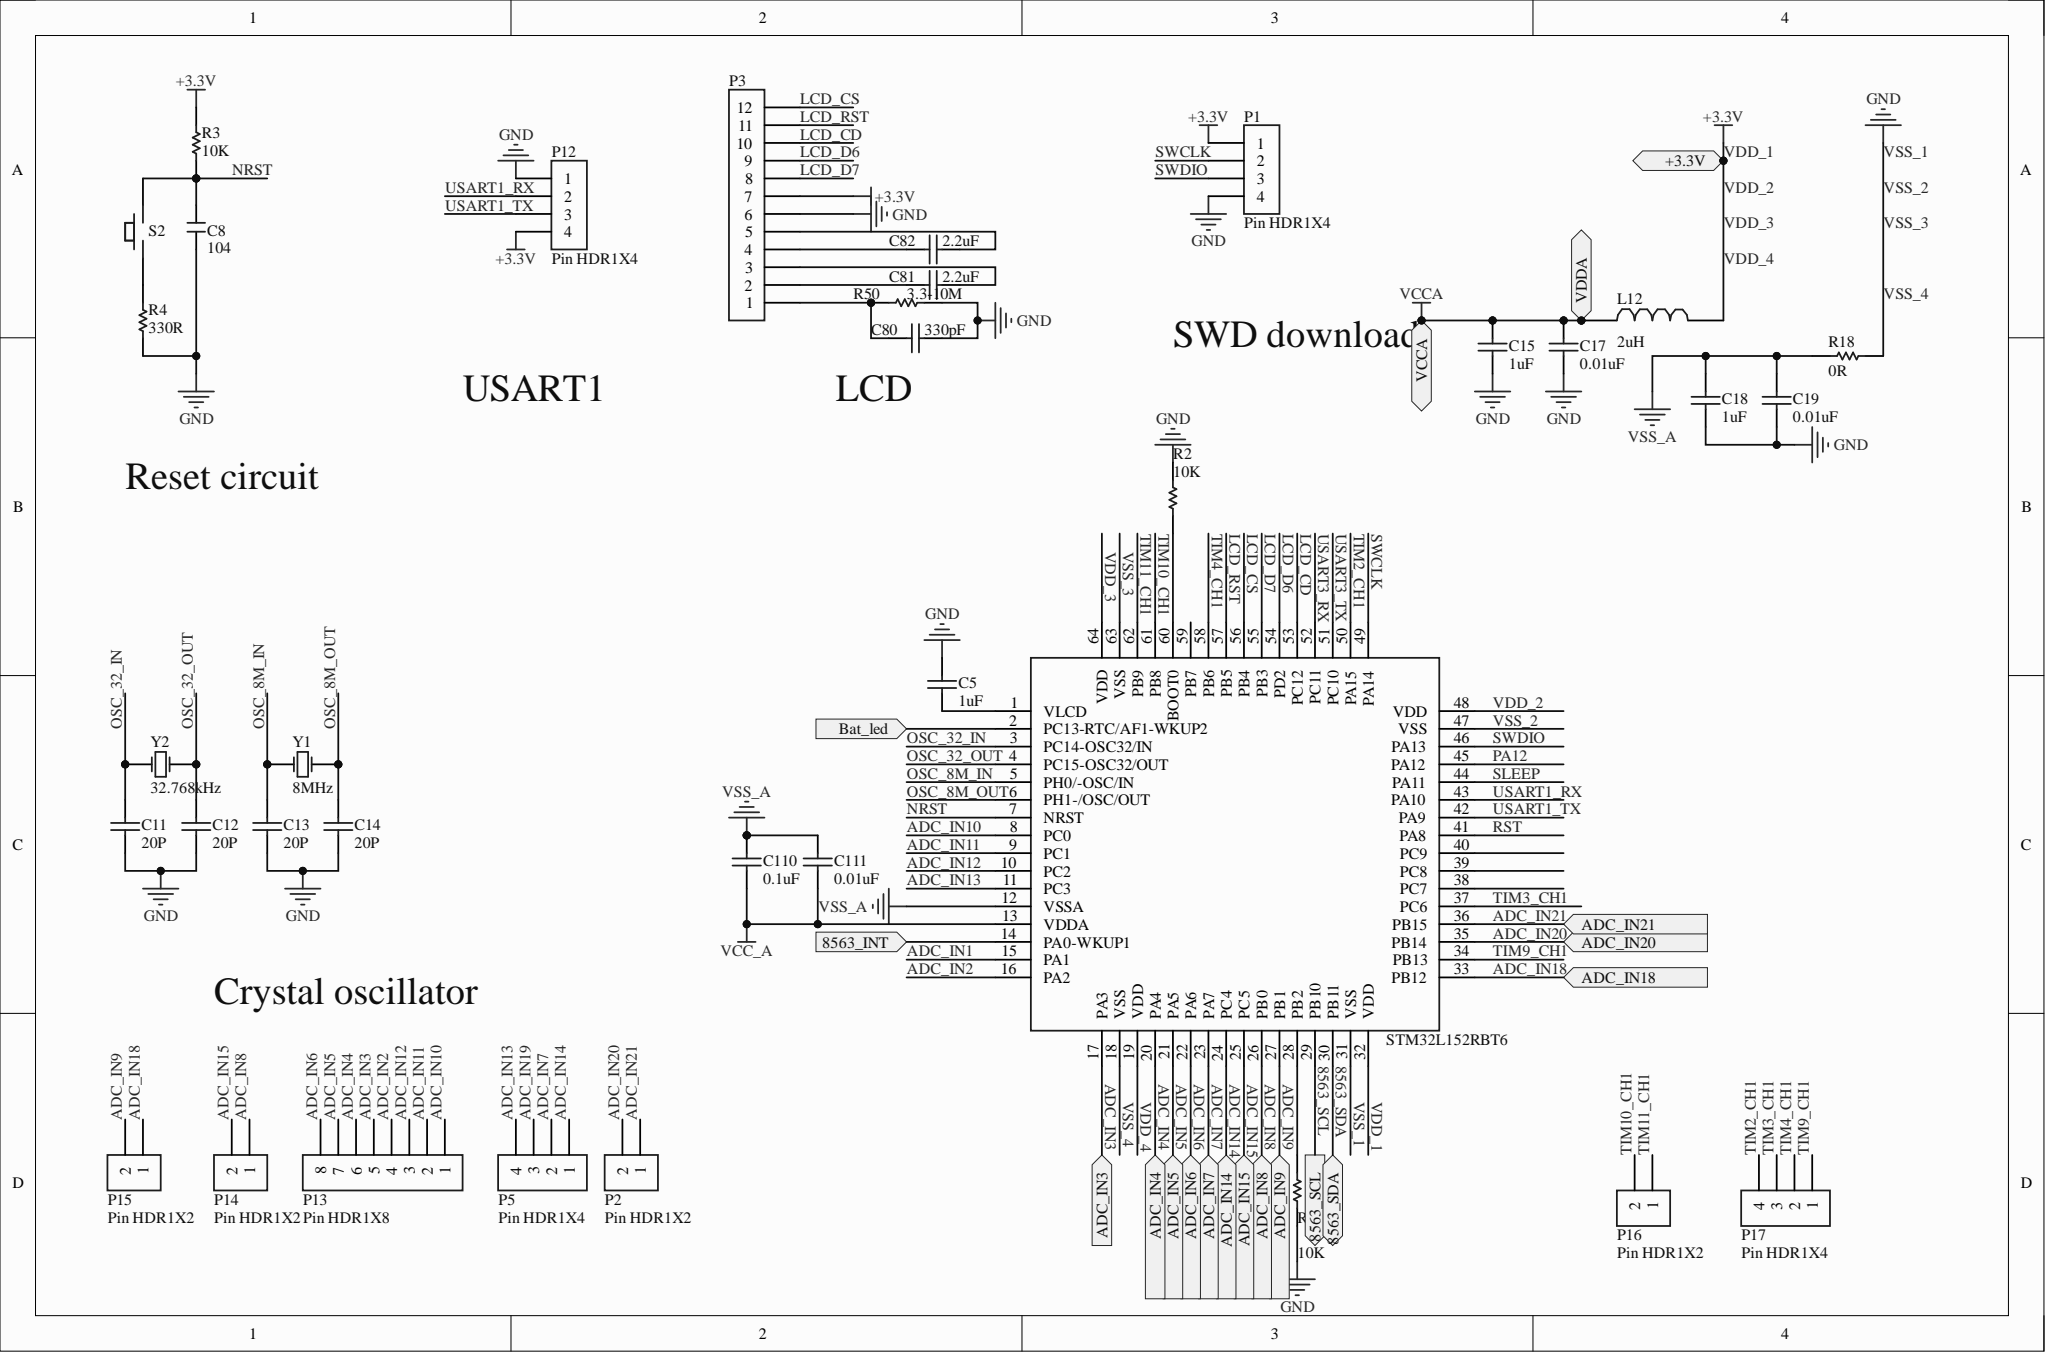Circuit board | Altium Designer | 36 parts | 51 nets
Bill of materials:
Comment,Description,Designator,Footprint,LibRef,Quantity
"1uF","Capacitor","C5, C15, C18","C 0603","C_1","3"
"104","Non-polar chip capacitor","C8","C 0603","C","1"
"20P","Capacitor","C11, C12, C13, C14","C 0603","C_2, C_1","4"
"0.01uF","Capacitor","C17, C19, C111","C 0603","C_1, C_3","3"
"330pF","Capacitor","C80","C 0603","C_1","1"
"2.2uF","Capacitor","C81, C82","C 0603","C_1","2"
"0.1uF","Capacitor","C110","C 0603","C_1","1"
"2uH","INDUCTOR","L12","R 0603","INDUCTOR","1"
"Pin HDR1X4","","P1, P5, P12, P17","Pin HDR1X4/2.54mm-S","Pin HDR1X4_1, Pin HDR1X4","4"
"Pin HDR1X2","","P2, P14, P15, P16","Pin HDR1X2/2.54mm-S","Pin HDR1X2","4"
"Pin HDR1X12","","P3","Pin HDR1X12/2.54mm-S","Pin HDR1X12","1"
"Pin HDR1X8","","P13","Pin HDR1X8/2.54mm-S","Pin HDR1X8","1"
"10K","Resistor","R1, R2, R3","0603R","RES0603","3"
"330R","Resistor","R4","0603R","RES0603_1","1"
"0R","Resistor","R18","0603R","RES0603","1"
"3.3-10M","Resistor","R50","0603R","RES0603_2","1"
"KEY","Ordinary tactile button","S2","SWTP3.7X6","KEY","1"
"STM32L152RBT6","","U1","LQFP-64_L10.0-W10.0-P0.50-LS12.0-BL","STM32L152RBT6","1"
"8MHz","Crystal Oscillator","Y1","XTAL_SMD49S","XTAL","1"
"32.768kHz","Crystal Oscillator","Y2","OSC 3215-2P","XTAL_1","1"
Netlist (Protel format):
[
C5
C 0603
1uF



]
[
C8
C 0603
104



]
[
C11
C 0603
20P



]
[
C12
C 0603
20P



]
[
C13
C 0603
20P



]
[
C14
C 0603
20P



]
[
C15
C 0603
1uF



]
[
C17
C 0603
0.01uF



]
[
C18
C 0603
1uF



]
[
C19
C 0603
0.01uF



]
[
C80
C 0603
330pF



]
[
C81
C 0603
2.2uF



]
[
C82
C 0603
2.2uF



]
[
C110
C 0603
0.1uF



]
[
C111
C 0603
0.01uF



]
[
L12
R 0603
2uH



]
[
P1
Pin HDR1X4/2.54mm-S
Pin HDR1X4



]
[
P2
Pin HDR1X2/2.54mm-S
Pin HDR1X2



]
[
P3
Pin HDR1X12/2.54mm-S
Pin HDR1X12



]
[
P5
Pin HDR1X4/2.54mm-S
Pin HDR1X4



]
[
P12
Pin HDR1X4/2.54mm-S
Pin HDR1X4



]
[
P13
Pin HDR1X8/2.54mm-S
Pin HDR1X8



]
[
P14
Pin HDR1X2/2.54mm-S
Pin HDR1X2



]
[
P15
Pin HDR1X2/2.54mm-S
Pin HDR1X2



]
[
P16
Pin HDR1X2/2.54mm-S
Pin HDR1X2



]
[
P17
Pin HDR1X4/2.54mm-S
Pin HDR1X4



]
[
R1
0603R
10K



]
[
R2
0603R
10K



]
[
R3
0603R
10K



]
[
R4
0603R
330R



]
[
R18
0603R
0R



]
[
R50
0603R
3.3-10M



]
[
S2
SWTP3.7X6
KEY



]
[
U1
LQFP-64_L10.0-W10.0-P0.50-LS12.0-BL
STM32L152RBT6



]
[
Y1
XTAL_SMD49S
8MHz



]
[
Y2
OSC 3215-2P
32.768kHz



]
(
VSS_A
C18-2
C19-2
C110-1
C111-1
R18-2
U1-12
)
(
VSS_1
C5-1
C8-1
C11-1
C12-2
C13-1
C14-2
C15-1
C17-1
C18-1
C19-1
C80-2
P1-4
P3-6
P12-1
R1-1
R2-2
R4-1
R18-1
R50-1
U1-18
U1-31
U1-47
U1-63
)
(
VDD_1
L12-2
P1-1
P3-7
P12-4
R3-2
U1-19
U1-32
U1-48
U1-64
)
(
VCCA
C15-2
C17-2
L12-1
)
(
VCC_A
C110-2
C111-2
U1-13
)
(
USART1_TX
P12-3
U1-42
)
(
USART1_RX
P12-2
U1-43
)
(
TIM11_CH1
P16-1
U1-62
)
(
TIM10_CH1
P16-2
U1-61
)
(
TIM9_CH1
P17-1
U1-34
)
(
TIM4_CH1
P17-2
U1-58
)
(
TIM3_CH1
P17-3
U1-37
)
(
TIM2_CH1
P17-4
U1-50
)
(
SWDIO
P1-3
U1-46
)
(
SWCLK
P1-2
U1-49
)
(
OSC_32_OUT
C12-1
U1-4
Y2-2
)
(
OSC_32_IN
C11-2
U1-3
Y2-1
)
(
OSC_8M_OUT
C14-1
U1-6
Y1-1
)
(
OSC_8M_IN
C13-2
U1-5
Y1-2
)
(
NRST
C8-2
R3-1
S2-2
U1-7
)
(
NetR4_2
R4-2
S2-1
)
(
NetR2_1
R2-1
U1-60
)
(
NetR1_2
R1-2
U1-28
)
(
NetC82_2
C82-2
P3-5
)
(
NetC82_1
C82-1
P3-4
)
(
NetC81_2
C81-2
P3-3
)
(
NetC81_1
C81-1
P3-2
)
(
NetC80_1
C80-1
P3-1
R50-2
)
(
NetC5_2
C5-2
U1-1
)
(
LCD_RST
P3-11
U1-57
)
(
LCD_D7
P3-8
U1-55
)
(
LCD_D6
P3-9
U1-54
)
(
LCD_CS
P3-12
U1-56
)
(
LCD_CD
P3-10
U1-53
)
(
ADC_IN21
P2-1
U1-36
)
(
ADC_IN20
P2-2
U1-35
)
(
ADC_IN18
P15-1
U1-33
)
(
ADC_IN15
P14-2
U1-25
)
(
ADC_IN14
P5-1
U1-24
)
(
ADC_IN13
P5-4
U1-11
)
(
ADC_IN12
P13-3
U1-10
)
(
ADC_IN11
P13-2
U1-9
)
(
ADC_IN10
P13-1
U1-8
)
(
ADC_IN9
P15-2
U1-27
)
(
ADC_IN8
P14-1
U1-26
)
(
ADC_IN7
P5-2
U1-23
)
(
ADC_IN6
P13-8
U1-22
)
(
ADC_IN5
P13-7
U1-21
)
(
ADC_IN4
P13-6
U1-20
)
(
ADC_IN3
P13-5
U1-17
)
(
ADC_IN2
P13-4
U1-16
)